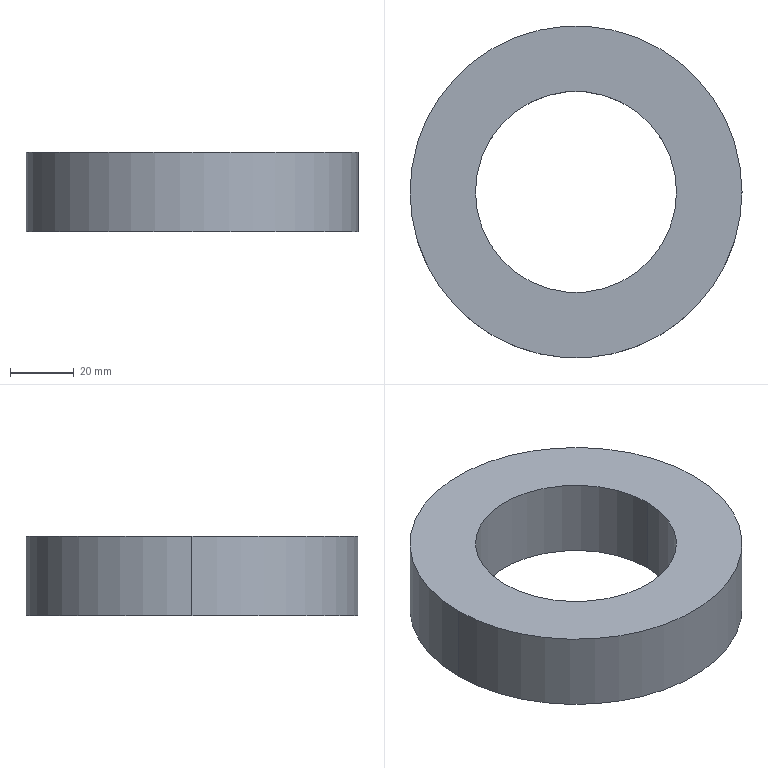Part | STEP file | FERRIITI_104 | 1 solid | 6 faces | box 104 x 104 x 25 mm | volume 134441 mm3 | cylinder 4 | plane 2 | commonest cylinder face diameters 63 x2 104 x2
STEP:
#1=CARTESIAN_POINT('',(0.,0.,0.));
#2=DIRECTION('',(0.,0.,1.));
#3=DIRECTION('',(1.,0.,0.));
#4=AXIS2_PLACEMENT_3D('',#1,#2,#3);
#5=CARTESIAN_POINT('',(52.,0.,0.));
#6=VERTEX_POINT('',#5);
#7=CARTESIAN_POINT('',(-52.,0.,0.));
#8=VERTEX_POINT('',#7);
#9=CARTESIAN_POINT('',(0.,0.,0.));
#10=DIRECTION('',(0.,0.,1.));
#11=DIRECTION('',(1.,0.,0.));
#12=AXIS2_PLACEMENT_3D('',#9,#10,#11);
#13=CIRCLE('',#12,52.);
#14=CARTESIAN_POINT('',(0.,0.,0.));
#15=DIRECTION('',(0.,0.,1.));
#16=DIRECTION('',(1.,0.,0.));
#17=AXIS2_PLACEMENT_3D('',#14,#15,#16);
#18=PLANE('',#17);
#19=CARTESIAN_POINT('',(0.,0.));
#20=DIRECTION('',(1.,0.));
#21=AXIS2_PLACEMENT_2D('',#19,#20);
#22=CIRCLE('',#21,52.);
#23=(GEOMETRIC_REPRESENTATION_CONTEXT(2)PARAMETRIC_REPRESENTATION_CONTEXT()REPRESENTATION_CONTEXT('',''));
#24=DEFINITIONAL_REPRESENTATION('',(#22),#23);
#25=PCURVE('',#18,#24);
#26=CARTESIAN_POINT('',(0.,0.,0.));
#27=DIRECTION('',(0.,0.,1.));
#28=DIRECTION('',(1.,0.,0.));
#29=AXIS2_PLACEMENT_3D('',#26,#27,#28);
#30=CYLINDRICAL_SURFACE('',#29,52.);
#31=CARTESIAN_POINT('',(0.,0.));
#32=DIRECTION('',(1.,0.));
#33=VECTOR('',#32,1.);
#34=LINE('',#31,#33);
#35=(GEOMETRIC_REPRESENTATION_CONTEXT(2)PARAMETRIC_REPRESENTATION_CONTEXT()REPRESENTATION_CONTEXT('',''));
#36=DEFINITIONAL_REPRESENTATION('',(#34),#35);
#37=PCURVE('',#30,#36);
#38=SURFACE_CURVE('',#13,(#25,#37),.PCURVE_S1.);
#39=EDGE_CURVE('',#6,#8,#38,.T.);
#40=ORIENTED_EDGE('',*,*,#39,.T.);
#41=CARTESIAN_POINT('',(0.,0.,0.));
#42=DIRECTION('',(0.,0.,1.));
#43=DIRECTION('',(-1.,0.,0.));
#44=AXIS2_PLACEMENT_3D('',#41,#42,#43);
#45=CIRCLE('',#44,52.);
#46=CARTESIAN_POINT('',(0.,0.));
#47=DIRECTION('',(-1.,0.));
#48=AXIS2_PLACEMENT_2D('',#46,#47);
#49=CIRCLE('',#48,52.);
#50=(GEOMETRIC_REPRESENTATION_CONTEXT(2)PARAMETRIC_REPRESENTATION_CONTEXT()REPRESENTATION_CONTEXT('',''));
#51=DEFINITIONAL_REPRESENTATION('',(#49),#50);
#52=PCURVE('',#18,#51);
#53=CARTESIAN_POINT('',(0.,0.,0.));
#54=DIRECTION('',(0.,0.,1.));
#55=DIRECTION('',(1.,0.,0.));
#56=AXIS2_PLACEMENT_3D('',#53,#54,#55);
#57=CYLINDRICAL_SURFACE('',#56,52.);
#58=CARTESIAN_POINT('',(3.142,0.));
#59=DIRECTION('',(1.,0.));
#60=VECTOR('',#59,1.);
#61=LINE('',#58,#60);
#62=(GEOMETRIC_REPRESENTATION_CONTEXT(2)PARAMETRIC_REPRESENTATION_CONTEXT()REPRESENTATION_CONTEXT('',''));
#63=DEFINITIONAL_REPRESENTATION('',(#61),#62);
#64=PCURVE('',#57,#63);
#65=SURFACE_CURVE('',#45,(#52,#64),.PCURVE_S1.);
#66=EDGE_CURVE('',#8,#6,#65,.T.);
#67=ORIENTED_EDGE('',*,*,#66,.T.);
#68=EDGE_LOOP('',(#40,#67));
#69=FACE_BOUND('',#68,.F.);
#70=CARTESIAN_POINT('',(31.5,0.,0.));
#71=VERTEX_POINT('',#70);
#72=CARTESIAN_POINT('',(-31.5,0.,0.));
#73=VERTEX_POINT('',#72);
#74=CARTESIAN_POINT('',(0.,0.,0.));
#75=DIRECTION('',(0.,0.,1.));
#76=DIRECTION('',(1.,0.,0.));
#77=AXIS2_PLACEMENT_3D('',#74,#75,#76);
#78=CIRCLE('',#77,31.5);
#79=CARTESIAN_POINT('',(0.,0.));
#80=DIRECTION('',(1.,0.));
#81=AXIS2_PLACEMENT_2D('',#79,#80);
#82=CIRCLE('',#81,31.5);
#83=(GEOMETRIC_REPRESENTATION_CONTEXT(2)PARAMETRIC_REPRESENTATION_CONTEXT()REPRESENTATION_CONTEXT('',''));
#84=DEFINITIONAL_REPRESENTATION('',(#82),#83);
#85=PCURVE('',#18,#84);
#86=CARTESIAN_POINT('',(0.,0.,25.));
#87=DIRECTION('',(0.,0.,1.));
#88=DIRECTION('',(1.,0.,0.));
#89=AXIS2_PLACEMENT_3D('',#86,#87,#88);
#90=CYLINDRICAL_SURFACE('',#89,31.5);
#91=CARTESIAN_POINT('',(0.,-25.));
#92=DIRECTION('',(1.,0.));
#93=VECTOR('',#92,1.);
#94=LINE('',#91,#93);
#95=(GEOMETRIC_REPRESENTATION_CONTEXT(2)PARAMETRIC_REPRESENTATION_CONTEXT()REPRESENTATION_CONTEXT('',''));
#96=DEFINITIONAL_REPRESENTATION('',(#94),#95);
#97=PCURVE('',#90,#96);
#98=SURFACE_CURVE('',#78,(#85,#97),.PCURVE_S1.);
#99=EDGE_CURVE('',#71,#73,#98,.T.);
#100=ORIENTED_EDGE('',*,*,#99,.F.);
#101=CARTESIAN_POINT('',(0.,0.,0.));
#102=DIRECTION('',(0.,0.,1.));
#103=DIRECTION('',(-1.,0.,0.));
#104=AXIS2_PLACEMENT_3D('',#101,#102,#103);
#105=CIRCLE('',#104,31.5);
#106=CARTESIAN_POINT('',(0.,0.));
#107=DIRECTION('',(-1.,0.));
#108=AXIS2_PLACEMENT_2D('',#106,#107);
#109=CIRCLE('',#108,31.5);
#110=(GEOMETRIC_REPRESENTATION_CONTEXT(2)PARAMETRIC_REPRESENTATION_CONTEXT()REPRESENTATION_CONTEXT('',''));
#111=DEFINITIONAL_REPRESENTATION('',(#109),#110);
#112=PCURVE('',#18,#111);
#113=CARTESIAN_POINT('',(0.,0.,25.));
#114=DIRECTION('',(0.,0.,1.));
#115=DIRECTION('',(1.,0.,0.));
#116=AXIS2_PLACEMENT_3D('',#113,#114,#115);
#117=CYLINDRICAL_SURFACE('',#116,31.5);
#118=CARTESIAN_POINT('',(3.142,-25.));
#119=DIRECTION('',(1.,0.));
#120=VECTOR('',#119,1.);
#121=LINE('',#118,#120);
#122=(GEOMETRIC_REPRESENTATION_CONTEXT(2)PARAMETRIC_REPRESENTATION_CONTEXT()REPRESENTATION_CONTEXT('',''));
#123=DEFINITIONAL_REPRESENTATION('',(#121),#122);
#124=PCURVE('',#117,#123);
#125=SURFACE_CURVE('',#105,(#112,#124),.PCURVE_S1.);
#126=EDGE_CURVE('',#73,#71,#125,.T.);
#127=ORIENTED_EDGE('',*,*,#126,.F.);
#128=EDGE_LOOP('',(#100,#127));
#129=FACE_BOUND('',#128,.F.);
#130=ADVANCED_FACE('',(#69,#129),#18,.F.);
#131=CARTESIAN_POINT('',(-52.,0.,25.));
#132=VERTEX_POINT('',#131);
#133=CARTESIAN_POINT('',(-52.,0.,0.));
#134=DIRECTION('',(0.,0.,1.));
#135=VECTOR('',#134,1.);
#136=LINE('',#133,#135);
#137=CARTESIAN_POINT('',(3.142,0.));
#138=DIRECTION('',(0.,1.));
#139=VECTOR('',#138,1.);
#140=LINE('',#137,#139);
#141=(GEOMETRIC_REPRESENTATION_CONTEXT(2)PARAMETRIC_REPRESENTATION_CONTEXT()REPRESENTATION_CONTEXT('',''));
#142=DEFINITIONAL_REPRESENTATION('',(#140),#141);
#143=PCURVE('',#30,#142);
#144=CARTESIAN_POINT('',(3.142,0.));
#145=DIRECTION('',(0.,1.));
#146=VECTOR('',#145,1.);
#147=LINE('',#144,#146);
#148=(GEOMETRIC_REPRESENTATION_CONTEXT(2)PARAMETRIC_REPRESENTATION_CONTEXT()REPRESENTATION_CONTEXT('',''));
#149=DEFINITIONAL_REPRESENTATION('',(#147),#148);
#150=PCURVE('',#57,#149);
#151=SURFACE_CURVE('',#136,(#143,#150),.PCURVE_S1.);
#152=EDGE_CURVE('',#8,#132,#151,.T.);
#153=ORIENTED_EDGE('',*,*,#152,.T.);
#154=CARTESIAN_POINT('',(52.,0.,25.));
#155=VERTEX_POINT('',#154);
#156=CARTESIAN_POINT('',(0.,0.,25.));
#157=DIRECTION('',(0.,0.,1.));
#158=DIRECTION('',(1.,0.,0.));
#159=AXIS2_PLACEMENT_3D('',#156,#157,#158);
#160=CIRCLE('',#159,52.);
#161=CARTESIAN_POINT('',(0.,25.));
#162=DIRECTION('',(1.,0.));
#163=VECTOR('',#162,1.);
#164=LINE('',#161,#163);
#165=(GEOMETRIC_REPRESENTATION_CONTEXT(2)PARAMETRIC_REPRESENTATION_CONTEXT()REPRESENTATION_CONTEXT('',''));
#166=DEFINITIONAL_REPRESENTATION('',(#164),#165);
#167=PCURVE('',#30,#166);
#168=CARTESIAN_POINT('',(0.,0.,25.));
#169=DIRECTION('',(0.,0.,1.));
#170=DIRECTION('',(1.,0.,0.));
#171=AXIS2_PLACEMENT_3D('',#168,#169,#170);
#172=PLANE('',#171);
#173=CARTESIAN_POINT('',(0.,0.));
#174=DIRECTION('',(1.,0.));
#175=AXIS2_PLACEMENT_2D('',#173,#174);
#176=CIRCLE('',#175,52.);
#177=(GEOMETRIC_REPRESENTATION_CONTEXT(2)PARAMETRIC_REPRESENTATION_CONTEXT()REPRESENTATION_CONTEXT('',''));
#178=DEFINITIONAL_REPRESENTATION('',(#176),#177);
#179=PCURVE('',#172,#178);
#180=SURFACE_CURVE('',#160,(#167,#179),.PCURVE_S1.);
#181=EDGE_CURVE('',#155,#132,#180,.T.);
#182=ORIENTED_EDGE('',*,*,#181,.F.);
#183=CARTESIAN_POINT('',(52.,0.,0.));
#184=DIRECTION('',(0.,0.,1.));
#185=VECTOR('',#184,1.);
#186=LINE('',#183,#185);
#187=CARTESIAN_POINT('',(0.,0.));
#188=DIRECTION('',(0.,1.));
#189=VECTOR('',#188,1.);
#190=LINE('',#187,#189);
#191=(GEOMETRIC_REPRESENTATION_CONTEXT(2)PARAMETRIC_REPRESENTATION_CONTEXT()REPRESENTATION_CONTEXT('',''));
#192=DEFINITIONAL_REPRESENTATION('',(#190),#191);
#193=PCURVE('',#30,#192);
#194=CARTESIAN_POINT('',(6.283,0.));
#195=DIRECTION('',(0.,1.));
#196=VECTOR('',#195,1.);
#197=LINE('',#194,#196);
#198=(GEOMETRIC_REPRESENTATION_CONTEXT(2)PARAMETRIC_REPRESENTATION_CONTEXT()REPRESENTATION_CONTEXT('',''));
#199=DEFINITIONAL_REPRESENTATION('',(#197),#198);
#200=PCURVE('',#57,#199);
#201=SURFACE_CURVE('',#186,(#193,#200),.PCURVE_S1.);
#202=EDGE_CURVE('',#6,#155,#201,.T.);
#203=ORIENTED_EDGE('',*,*,#202,.F.);
#204=ORIENTED_EDGE('',*,*,#39,.T.);
#205=EDGE_LOOP('',(#153,#182,#203,#204));
#206=FACE_BOUND('',#205,.T.);
#207=ADVANCED_FACE('',(#206),#30,.T.);
#208=ORIENTED_EDGE('',*,*,#202,.T.);
#209=CARTESIAN_POINT('',(0.,0.,25.));
#210=DIRECTION('',(0.,0.,1.));
#211=DIRECTION('',(-1.,0.,0.));
#212=AXIS2_PLACEMENT_3D('',#209,#210,#211);
#213=CIRCLE('',#212,52.);
#214=CARTESIAN_POINT('',(3.142,25.));
#215=DIRECTION('',(1.,0.));
#216=VECTOR('',#215,1.);
#217=LINE('',#214,#216);
#218=(GEOMETRIC_REPRESENTATION_CONTEXT(2)PARAMETRIC_REPRESENTATION_CONTEXT()REPRESENTATION_CONTEXT('',''));
#219=DEFINITIONAL_REPRESENTATION('',(#217),#218);
#220=PCURVE('',#57,#219);
#221=CARTESIAN_POINT('',(0.,0.));
#222=DIRECTION('',(-1.,0.));
#223=AXIS2_PLACEMENT_2D('',#221,#222);
#224=CIRCLE('',#223,52.);
#225=(GEOMETRIC_REPRESENTATION_CONTEXT(2)PARAMETRIC_REPRESENTATION_CONTEXT()REPRESENTATION_CONTEXT('',''));
#226=DEFINITIONAL_REPRESENTATION('',(#224),#225);
#227=PCURVE('',#172,#226);
#228=SURFACE_CURVE('',#213,(#220,#227),.PCURVE_S1.);
#229=EDGE_CURVE('',#132,#155,#228,.T.);
#230=ORIENTED_EDGE('',*,*,#229,.F.);
#231=ORIENTED_EDGE('',*,*,#152,.F.);
#232=ORIENTED_EDGE('',*,*,#66,.T.);
#233=EDGE_LOOP('',(#208,#230,#231,#232));
#234=FACE_BOUND('',#233,.T.);
#235=ADVANCED_FACE('',(#234),#57,.T.);
#236=ORIENTED_EDGE('',*,*,#181,.F.);
#237=ORIENTED_EDGE('',*,*,#229,.F.);
#238=EDGE_LOOP('',(#236,#237));
#239=FACE_BOUND('',#238,.F.);
#240=CARTESIAN_POINT('',(31.5,0.,25.));
#241=VERTEX_POINT('',#240);
#242=CARTESIAN_POINT('',(-31.5,0.,25.));
#243=VERTEX_POINT('',#242);
#244=CARTESIAN_POINT('',(0.,0.,25.));
#245=DIRECTION('',(0.,0.,1.));
#246=DIRECTION('',(1.,0.,0.));
#247=AXIS2_PLACEMENT_3D('',#244,#245,#246);
#248=CIRCLE('',#247,31.5);
#249=CARTESIAN_POINT('',(0.,0.));
#250=DIRECTION('',(1.,0.));
#251=AXIS2_PLACEMENT_2D('',#249,#250);
#252=CIRCLE('',#251,31.5);
#253=(GEOMETRIC_REPRESENTATION_CONTEXT(2)PARAMETRIC_REPRESENTATION_CONTEXT()REPRESENTATION_CONTEXT('',''));
#254=DEFINITIONAL_REPRESENTATION('',(#252),#253);
#255=PCURVE('',#172,#254);
#256=CARTESIAN_POINT('',(0.,0.));
#257=DIRECTION('',(1.,0.));
#258=VECTOR('',#257,1.);
#259=LINE('',#256,#258);
#260=(GEOMETRIC_REPRESENTATION_CONTEXT(2)PARAMETRIC_REPRESENTATION_CONTEXT()REPRESENTATION_CONTEXT('',''));
#261=DEFINITIONAL_REPRESENTATION('',(#259),#260);
#262=PCURVE('',#90,#261);
#263=SURFACE_CURVE('',#248,(#255,#262),.PCURVE_S1.);
#264=EDGE_CURVE('',#241,#243,#263,.T.);
#265=ORIENTED_EDGE('',*,*,#264,.T.);
#266=CARTESIAN_POINT('',(0.,0.,25.));
#267=DIRECTION('',(0.,0.,1.));
#268=DIRECTION('',(-1.,0.,0.));
#269=AXIS2_PLACEMENT_3D('',#266,#267,#268);
#270=CIRCLE('',#269,31.5);
#271=CARTESIAN_POINT('',(0.,0.));
#272=DIRECTION('',(-1.,0.));
#273=AXIS2_PLACEMENT_2D('',#271,#272);
#274=CIRCLE('',#273,31.5);
#275=(GEOMETRIC_REPRESENTATION_CONTEXT(2)PARAMETRIC_REPRESENTATION_CONTEXT()REPRESENTATION_CONTEXT('',''));
#276=DEFINITIONAL_REPRESENTATION('',(#274),#275);
#277=PCURVE('',#172,#276);
#278=CARTESIAN_POINT('',(3.142,0.));
#279=DIRECTION('',(1.,0.));
#280=VECTOR('',#279,1.);
#281=LINE('',#278,#280);
#282=(GEOMETRIC_REPRESENTATION_CONTEXT(2)PARAMETRIC_REPRESENTATION_CONTEXT()REPRESENTATION_CONTEXT('',''));
#283=DEFINITIONAL_REPRESENTATION('',(#281),#282);
#284=PCURVE('',#117,#283);
#285=SURFACE_CURVE('',#270,(#277,#284),.PCURVE_S1.);
#286=EDGE_CURVE('',#243,#241,#285,.T.);
#287=ORIENTED_EDGE('',*,*,#286,.T.);
#288=EDGE_LOOP('',(#265,#287));
#289=FACE_BOUND('',#288,.F.);
#290=ADVANCED_FACE('',(#239,#289),#172,.T.);
#291=ORIENTED_EDGE('',*,*,#99,.T.);
#292=CARTESIAN_POINT('',(-31.5,0.,25.));
#293=DIRECTION('',(0.,0.,-1.));
#294=VECTOR('',#293,1.);
#295=LINE('',#292,#294);
#296=CARTESIAN_POINT('',(3.142,0.));
#297=DIRECTION('',(0.,-1.));
#298=VECTOR('',#297,1.);
#299=LINE('',#296,#298);
#300=(GEOMETRIC_REPRESENTATION_CONTEXT(2)PARAMETRIC_REPRESENTATION_CONTEXT()REPRESENTATION_CONTEXT('',''));
#301=DEFINITIONAL_REPRESENTATION('',(#299),#300);
#302=PCURVE('',#90,#301);
#303=CARTESIAN_POINT('',(3.142,0.));
#304=DIRECTION('',(0.,-1.));
#305=VECTOR('',#304,1.);
#306=LINE('',#303,#305);
#307=(GEOMETRIC_REPRESENTATION_CONTEXT(2)PARAMETRIC_REPRESENTATION_CONTEXT()REPRESENTATION_CONTEXT('',''));
#308=DEFINITIONAL_REPRESENTATION('',(#306),#307);
#309=PCURVE('',#117,#308);
#310=SURFACE_CURVE('',#295,(#302,#309),.PCURVE_S1.);
#311=EDGE_CURVE('',#243,#73,#310,.T.);
#312=ORIENTED_EDGE('',*,*,#311,.F.);
#313=ORIENTED_EDGE('',*,*,#264,.F.);
#314=CARTESIAN_POINT('',(31.5,0.,25.));
#315=DIRECTION('',(0.,0.,-1.));
#316=VECTOR('',#315,1.);
#317=LINE('',#314,#316);
#318=CARTESIAN_POINT('',(0.,0.));
#319=DIRECTION('',(0.,-1.));
#320=VECTOR('',#319,1.);
#321=LINE('',#318,#320);
#322=(GEOMETRIC_REPRESENTATION_CONTEXT(2)PARAMETRIC_REPRESENTATION_CONTEXT()REPRESENTATION_CONTEXT('',''));
#323=DEFINITIONAL_REPRESENTATION('',(#321),#322);
#324=PCURVE('',#90,#323);
#325=CARTESIAN_POINT('',(6.283,0.));
#326=DIRECTION('',(0.,-1.));
#327=VECTOR('',#326,1.);
#328=LINE('',#325,#327);
#329=(GEOMETRIC_REPRESENTATION_CONTEXT(2)PARAMETRIC_REPRESENTATION_CONTEXT()REPRESENTATION_CONTEXT('',''));
#330=DEFINITIONAL_REPRESENTATION('',(#328),#329);
#331=PCURVE('',#117,#330);
#332=SURFACE_CURVE('',#317,(#324,#331),.PCURVE_S1.);
#333=EDGE_CURVE('',#241,#71,#332,.T.);
#334=ORIENTED_EDGE('',*,*,#333,.T.);
#335=EDGE_LOOP('',(#291,#312,#313,#334));
#336=FACE_BOUND('',#335,.F.);
#337=ADVANCED_FACE('',(#336),#90,.F.);
#338=ORIENTED_EDGE('',*,*,#126,.T.);
#339=ORIENTED_EDGE('',*,*,#333,.F.);
#340=ORIENTED_EDGE('',*,*,#286,.F.);
#341=ORIENTED_EDGE('',*,*,#311,.T.);
#342=EDGE_LOOP('',(#338,#339,#340,#341));
#343=FACE_BOUND('',#342,.F.);
#344=ADVANCED_FACE('',(#343),#117,.F.);
#345=CLOSED_SHELL('',(#130,#207,#235,#290,#337,#344));
#346=MANIFOLD_SOLID_BREP('',#345);
#347=(LENGTH_UNIT()NAMED_UNIT(*)SI_UNIT(.MILLI.,.METRE.));
#348=UNCERTAINTY_MEASURE_WITH_UNIT(LENGTH_MEASURE(0.0000001),#347,'','');
#349=(NAMED_UNIT(*)PLANE_ANGLE_UNIT()SI_UNIT($,.RADIAN.));
#350=(NAMED_UNIT(*)SI_UNIT($,.STERADIAN.)SOLID_ANGLE_UNIT());
#351=(GEOMETRIC_REPRESENTATION_CONTEXT(3)GLOBAL_UNCERTAINTY_ASSIGNED_CONTEXT((#348))GLOBAL_UNIT_ASSIGNED_CONTEXT((#347,#349,#350))REPRESENTATION_CONTEXT('',''));
#352=ADVANCED_BREP_SHAPE_REPRESENTATION('',(#4,#346),#351);